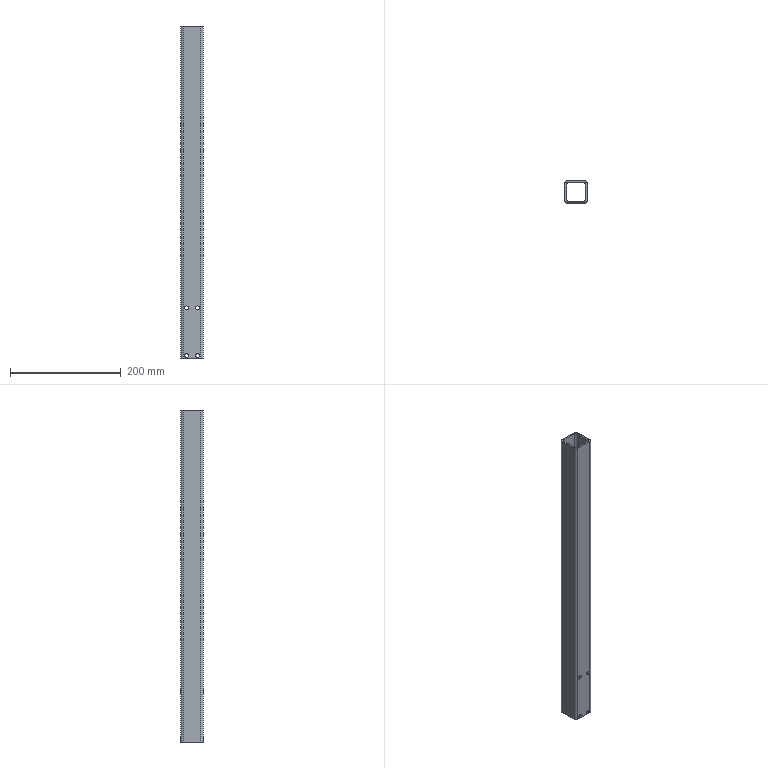Part | STEP file | DIN EN 10210-2 - 20 x 20 x 2 - 900 | 1 solid | 26 faces | box 40 x 40 x 600 mm | volume 259682 mm3 | cylinder 16 | plane 10 | commonest cylinder face diameters 7 x8 6 x4 9 x4